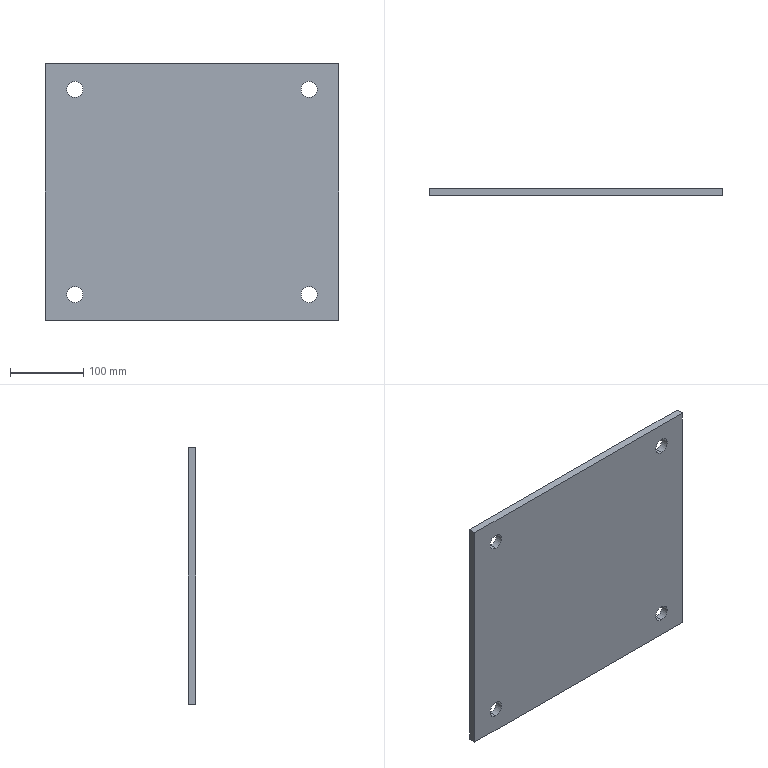Part | STEP file | 立柱Pad-400×350 | 1 solid | 14 faces | box 400 x 10 x 350 mm | volume 1384795 mm3 | cylinder 8 | plane 6 | commonest cylinder face diameters 22 x8
STEP:
#1=CARTESIAN_POINT('',(0.,0.,0.));
#2=DIRECTION('',(0.,0.,1.));
#3=DIRECTION('',(1.,0.,0.));
#4=AXIS2_PLACEMENT_3D('',#1,#2,#3);
#5=CARTESIAN_POINT('',(-160.,0.,-129.));
#6=VERTEX_POINT('',#5);
#7=CARTESIAN_POINT('',(-160.,10.,-129.));
#8=VERTEX_POINT('',#7);
#9=CARTESIAN_POINT('',(-160.,10.,-129.));
#10=DIRECTION('',(0.,1.,0.));
#11=VECTOR('',#10,1.);
#12=LINE('',#9,#11);
#13=CARTESIAN_POINT('',(-160.,10.,-140.));
#14=DIRECTION('',(0.,1.,0.));
#15=DIRECTION('',(0.,0.,1.));
#16=AXIS2_PLACEMENT_3D('',#13,#14,#15);
#17=CYLINDRICAL_SURFACE('',#16,11.);
#18=CARTESIAN_POINT('',(6.283,0.));
#19=DIRECTION('',(0.,1.));
#20=VECTOR('',#19,1.);
#21=LINE('',#18,#20);
#22=(GEOMETRIC_REPRESENTATION_CONTEXT(2)PARAMETRIC_REPRESENTATION_CONTEXT()REPRESENTATION_CONTEXT('',''));
#23=DEFINITIONAL_REPRESENTATION('',(#21),#22);
#24=PCURVE('',#17,#23);
#25=CARTESIAN_POINT('',(-160.,10.,-140.));
#26=DIRECTION('',(0.,1.,0.));
#27=DIRECTION('',(0.,0.,1.));
#28=AXIS2_PLACEMENT_3D('',#25,#26,#27);
#29=CYLINDRICAL_SURFACE('',#28,11.);
#30=CARTESIAN_POINT('',(0.,0.));
#31=DIRECTION('',(0.,1.));
#32=VECTOR('',#31,1.);
#33=LINE('',#30,#32);
#34=(GEOMETRIC_REPRESENTATION_CONTEXT(2)PARAMETRIC_REPRESENTATION_CONTEXT()REPRESENTATION_CONTEXT('',''));
#35=DEFINITIONAL_REPRESENTATION('',(#33),#34);
#36=PCURVE('',#29,#35);
#37=SURFACE_CURVE('',#12,(#24,#36),.PCURVE_S1.);
#38=EDGE_CURVE('',#6,#8,#37,.T.);
#39=ORIENTED_EDGE('',*,*,#38,.T.);
#40=CARTESIAN_POINT('',(-160.,10.,-151.));
#41=VERTEX_POINT('',#40);
#42=CARTESIAN_POINT('',(-160.,10.,-140.));
#43=DIRECTION('',(0.,1.,0.));
#44=DIRECTION('',(0.,0.,1.));
#45=AXIS2_PLACEMENT_3D('',#42,#43,#44);
#46=CIRCLE('',#45,11.);
#47=CARTESIAN_POINT('',(0.,0.));
#48=DIRECTION('',(1.,0.));
#49=VECTOR('',#48,1.);
#50=LINE('',#47,#49);
#51=(GEOMETRIC_REPRESENTATION_CONTEXT(2)PARAMETRIC_REPRESENTATION_CONTEXT()REPRESENTATION_CONTEXT('',''));
#52=DEFINITIONAL_REPRESENTATION('',(#50),#51);
#53=PCURVE('',#17,#52);
#54=CARTESIAN_POINT('',(0.,10.,0.));
#55=DIRECTION('',(0.,1.,0.));
#56=DIRECTION('',(0.,0.,1.));
#57=AXIS2_PLACEMENT_3D('',#54,#55,#56);
#58=PLANE('',#57);
#59=CARTESIAN_POINT('',(-140.,-160.));
#60=DIRECTION('',(1.,0.));
#61=AXIS2_PLACEMENT_2D('',#59,#60);
#62=CIRCLE('',#61,11.);
#63=(GEOMETRIC_REPRESENTATION_CONTEXT(2)PARAMETRIC_REPRESENTATION_CONTEXT()REPRESENTATION_CONTEXT('',''));
#64=DEFINITIONAL_REPRESENTATION('',(#62),#63);
#65=PCURVE('',#58,#64);
#66=SURFACE_CURVE('',#46,(#53,#65),.PCURVE_S1.);
#67=EDGE_CURVE('',#41,#8,#66,.T.);
#68=ORIENTED_EDGE('',*,*,#67,.F.);
#69=CARTESIAN_POINT('',(-160.,0.,-151.));
#70=VERTEX_POINT('',#69);
#71=CARTESIAN_POINT('',(-160.,10.,-151.));
#72=DIRECTION('',(0.,1.,0.));
#73=VECTOR('',#72,1.);
#74=LINE('',#71,#73);
#75=CARTESIAN_POINT('',(3.142,0.));
#76=DIRECTION('',(0.,1.));
#77=VECTOR('',#76,1.);
#78=LINE('',#75,#77);
#79=(GEOMETRIC_REPRESENTATION_CONTEXT(2)PARAMETRIC_REPRESENTATION_CONTEXT()REPRESENTATION_CONTEXT('',''));
#80=DEFINITIONAL_REPRESENTATION('',(#78),#79);
#81=PCURVE('',#17,#80);
#82=CARTESIAN_POINT('',(3.142,0.));
#83=DIRECTION('',(0.,1.));
#84=VECTOR('',#83,1.);
#85=LINE('',#82,#84);
#86=(GEOMETRIC_REPRESENTATION_CONTEXT(2)PARAMETRIC_REPRESENTATION_CONTEXT()REPRESENTATION_CONTEXT('',''));
#87=DEFINITIONAL_REPRESENTATION('',(#85),#86);
#88=PCURVE('',#29,#87);
#89=SURFACE_CURVE('',#74,(#81,#88),.PCURVE_S1.);
#90=EDGE_CURVE('',#70,#41,#89,.T.);
#91=ORIENTED_EDGE('',*,*,#90,.F.);
#92=CARTESIAN_POINT('',(-160.,0.,-140.));
#93=DIRECTION('',(0.,1.,0.));
#94=DIRECTION('',(0.,0.,1.));
#95=AXIS2_PLACEMENT_3D('',#92,#93,#94);
#96=CIRCLE('',#95,11.);
#97=CARTESIAN_POINT('',(0.,-10.));
#98=DIRECTION('',(1.,0.));
#99=VECTOR('',#98,1.);
#100=LINE('',#97,#99);
#101=(GEOMETRIC_REPRESENTATION_CONTEXT(2)PARAMETRIC_REPRESENTATION_CONTEXT()REPRESENTATION_CONTEXT('',''));
#102=DEFINITIONAL_REPRESENTATION('',(#100),#101);
#103=PCURVE('',#17,#102);
#104=CARTESIAN_POINT('',(0.,0.,0.));
#105=DIRECTION('',(0.,1.,0.));
#106=DIRECTION('',(0.,0.,1.));
#107=AXIS2_PLACEMENT_3D('',#104,#105,#106);
#108=PLANE('',#107);
#109=CARTESIAN_POINT('',(-140.,-160.));
#110=DIRECTION('',(1.,0.));
#111=AXIS2_PLACEMENT_2D('',#109,#110);
#112=CIRCLE('',#111,11.);
#113=(GEOMETRIC_REPRESENTATION_CONTEXT(2)PARAMETRIC_REPRESENTATION_CONTEXT()REPRESENTATION_CONTEXT('',''));
#114=DEFINITIONAL_REPRESENTATION('',(#112),#113);
#115=PCURVE('',#108,#114);
#116=SURFACE_CURVE('',#96,(#103,#115),.PCURVE_S1.);
#117=EDGE_CURVE('',#70,#6,#116,.T.);
#118=ORIENTED_EDGE('',*,*,#117,.T.);
#119=EDGE_LOOP('',(#39,#68,#91,#118));
#120=FACE_BOUND('',#119,.F.);
#121=ADVANCED_FACE('',(#120),#17,.F.);
#122=CARTESIAN_POINT('',(-160.,0.,151.));
#123=VERTEX_POINT('',#122);
#124=CARTESIAN_POINT('',(-160.,10.,151.));
#125=VERTEX_POINT('',#124);
#126=CARTESIAN_POINT('',(-160.,10.,151.));
#127=DIRECTION('',(0.,1.,0.));
#128=VECTOR('',#127,1.);
#129=LINE('',#126,#128);
#130=CARTESIAN_POINT('',(-160.,10.,140.));
#131=DIRECTION('',(0.,1.,0.));
#132=DIRECTION('',(0.,0.,1.));
#133=AXIS2_PLACEMENT_3D('',#130,#131,#132);
#134=CYLINDRICAL_SURFACE('',#133,11.);
#135=CARTESIAN_POINT('',(6.283,0.));
#136=DIRECTION('',(0.,1.));
#137=VECTOR('',#136,1.);
#138=LINE('',#135,#137);
#139=(GEOMETRIC_REPRESENTATION_CONTEXT(2)PARAMETRIC_REPRESENTATION_CONTEXT()REPRESENTATION_CONTEXT('',''));
#140=DEFINITIONAL_REPRESENTATION('',(#138),#139);
#141=PCURVE('',#134,#140);
#142=CARTESIAN_POINT('',(-160.,10.,140.));
#143=DIRECTION('',(0.,1.,0.));
#144=DIRECTION('',(0.,0.,1.));
#145=AXIS2_PLACEMENT_3D('',#142,#143,#144);
#146=CYLINDRICAL_SURFACE('',#145,11.);
#147=CARTESIAN_POINT('',(0.,0.));
#148=DIRECTION('',(0.,1.));
#149=VECTOR('',#148,1.);
#150=LINE('',#147,#149);
#151=(GEOMETRIC_REPRESENTATION_CONTEXT(2)PARAMETRIC_REPRESENTATION_CONTEXT()REPRESENTATION_CONTEXT('',''));
#152=DEFINITIONAL_REPRESENTATION('',(#150),#151);
#153=PCURVE('',#146,#152);
#154=SURFACE_CURVE('',#129,(#141,#153),.PCURVE_S1.);
#155=EDGE_CURVE('',#123,#125,#154,.T.);
#156=ORIENTED_EDGE('',*,*,#155,.T.);
#157=CARTESIAN_POINT('',(-160.,10.,129.));
#158=VERTEX_POINT('',#157);
#159=CARTESIAN_POINT('',(-160.,10.,140.));
#160=DIRECTION('',(0.,1.,0.));
#161=DIRECTION('',(0.,0.,1.));
#162=AXIS2_PLACEMENT_3D('',#159,#160,#161);
#163=CIRCLE('',#162,11.);
#164=CARTESIAN_POINT('',(0.,0.));
#165=DIRECTION('',(1.,0.));
#166=VECTOR('',#165,1.);
#167=LINE('',#164,#166);
#168=(GEOMETRIC_REPRESENTATION_CONTEXT(2)PARAMETRIC_REPRESENTATION_CONTEXT()REPRESENTATION_CONTEXT('',''));
#169=DEFINITIONAL_REPRESENTATION('',(#167),#168);
#170=PCURVE('',#134,#169);
#171=CARTESIAN_POINT('',(140.,-160.));
#172=DIRECTION('',(1.,0.));
#173=AXIS2_PLACEMENT_2D('',#171,#172);
#174=CIRCLE('',#173,11.);
#175=(GEOMETRIC_REPRESENTATION_CONTEXT(2)PARAMETRIC_REPRESENTATION_CONTEXT()REPRESENTATION_CONTEXT('',''));
#176=DEFINITIONAL_REPRESENTATION('',(#174),#175);
#177=PCURVE('',#58,#176);
#178=SURFACE_CURVE('',#163,(#170,#177),.PCURVE_S1.);
#179=EDGE_CURVE('',#158,#125,#178,.T.);
#180=ORIENTED_EDGE('',*,*,#179,.F.);
#181=CARTESIAN_POINT('',(-160.,0.,129.));
#182=VERTEX_POINT('',#181);
#183=CARTESIAN_POINT('',(-160.,10.,129.));
#184=DIRECTION('',(0.,1.,0.));
#185=VECTOR('',#184,1.);
#186=LINE('',#183,#185);
#187=CARTESIAN_POINT('',(3.142,0.));
#188=DIRECTION('',(0.,1.));
#189=VECTOR('',#188,1.);
#190=LINE('',#187,#189);
#191=(GEOMETRIC_REPRESENTATION_CONTEXT(2)PARAMETRIC_REPRESENTATION_CONTEXT()REPRESENTATION_CONTEXT('',''));
#192=DEFINITIONAL_REPRESENTATION('',(#190),#191);
#193=PCURVE('',#134,#192);
#194=CARTESIAN_POINT('',(3.142,0.));
#195=DIRECTION('',(0.,1.));
#196=VECTOR('',#195,1.);
#197=LINE('',#194,#196);
#198=(GEOMETRIC_REPRESENTATION_CONTEXT(2)PARAMETRIC_REPRESENTATION_CONTEXT()REPRESENTATION_CONTEXT('',''));
#199=DEFINITIONAL_REPRESENTATION('',(#197),#198);
#200=PCURVE('',#146,#199);
#201=SURFACE_CURVE('',#186,(#193,#200),.PCURVE_S1.);
#202=EDGE_CURVE('',#182,#158,#201,.T.);
#203=ORIENTED_EDGE('',*,*,#202,.F.);
#204=CARTESIAN_POINT('',(-160.,0.,140.));
#205=DIRECTION('',(0.,1.,0.));
#206=DIRECTION('',(0.,0.,1.));
#207=AXIS2_PLACEMENT_3D('',#204,#205,#206);
#208=CIRCLE('',#207,11.);
#209=CARTESIAN_POINT('',(0.,-10.));
#210=DIRECTION('',(1.,0.));
#211=VECTOR('',#210,1.);
#212=LINE('',#209,#211);
#213=(GEOMETRIC_REPRESENTATION_CONTEXT(2)PARAMETRIC_REPRESENTATION_CONTEXT()REPRESENTATION_CONTEXT('',''));
#214=DEFINITIONAL_REPRESENTATION('',(#212),#213);
#215=PCURVE('',#134,#214);
#216=CARTESIAN_POINT('',(140.,-160.));
#217=DIRECTION('',(1.,0.));
#218=AXIS2_PLACEMENT_2D('',#216,#217);
#219=CIRCLE('',#218,11.);
#220=(GEOMETRIC_REPRESENTATION_CONTEXT(2)PARAMETRIC_REPRESENTATION_CONTEXT()REPRESENTATION_CONTEXT('',''));
#221=DEFINITIONAL_REPRESENTATION('',(#219),#220);
#222=PCURVE('',#108,#221);
#223=SURFACE_CURVE('',#208,(#215,#222),.PCURVE_S1.);
#224=EDGE_CURVE('',#182,#123,#223,.T.);
#225=ORIENTED_EDGE('',*,*,#224,.T.);
#226=EDGE_LOOP('',(#156,#180,#203,#225));
#227=FACE_BOUND('',#226,.F.);
#228=ADVANCED_FACE('',(#227),#134,.F.);
#229=CARTESIAN_POINT('',(160.,0.,151.));
#230=VERTEX_POINT('',#229);
#231=CARTESIAN_POINT('',(160.,10.,151.));
#232=VERTEX_POINT('',#231);
#233=CARTESIAN_POINT('',(160.,10.,151.));
#234=DIRECTION('',(0.,1.,0.));
#235=VECTOR('',#234,1.);
#236=LINE('',#233,#235);
#237=CARTESIAN_POINT('',(160.,10.,140.));
#238=DIRECTION('',(0.,1.,0.));
#239=DIRECTION('',(0.,0.,1.));
#240=AXIS2_PLACEMENT_3D('',#237,#238,#239);
#241=CYLINDRICAL_SURFACE('',#240,11.);
#242=CARTESIAN_POINT('',(6.283,0.));
#243=DIRECTION('',(0.,1.));
#244=VECTOR('',#243,1.);
#245=LINE('',#242,#244);
#246=(GEOMETRIC_REPRESENTATION_CONTEXT(2)PARAMETRIC_REPRESENTATION_CONTEXT()REPRESENTATION_CONTEXT('',''));
#247=DEFINITIONAL_REPRESENTATION('',(#245),#246);
#248=PCURVE('',#241,#247);
#249=CARTESIAN_POINT('',(160.,10.,140.));
#250=DIRECTION('',(0.,1.,0.));
#251=DIRECTION('',(0.,0.,1.));
#252=AXIS2_PLACEMENT_3D('',#249,#250,#251);
#253=CYLINDRICAL_SURFACE('',#252,11.);
#254=CARTESIAN_POINT('',(0.,0.));
#255=DIRECTION('',(0.,1.));
#256=VECTOR('',#255,1.);
#257=LINE('',#254,#256);
#258=(GEOMETRIC_REPRESENTATION_CONTEXT(2)PARAMETRIC_REPRESENTATION_CONTEXT()REPRESENTATION_CONTEXT('',''));
#259=DEFINITIONAL_REPRESENTATION('',(#257),#258);
#260=PCURVE('',#253,#259);
#261=SURFACE_CURVE('',#236,(#248,#260),.PCURVE_S1.);
#262=EDGE_CURVE('',#230,#232,#261,.T.);
#263=ORIENTED_EDGE('',*,*,#262,.T.);
#264=CARTESIAN_POINT('',(160.,10.,129.));
#265=VERTEX_POINT('',#264);
#266=CARTESIAN_POINT('',(160.,10.,140.));
#267=DIRECTION('',(0.,1.,0.));
#268=DIRECTION('',(0.,0.,1.));
#269=AXIS2_PLACEMENT_3D('',#266,#267,#268);
#270=CIRCLE('',#269,11.);
#271=CARTESIAN_POINT('',(0.,0.));
#272=DIRECTION('',(1.,0.));
#273=VECTOR('',#272,1.);
#274=LINE('',#271,#273);
#275=(GEOMETRIC_REPRESENTATION_CONTEXT(2)PARAMETRIC_REPRESENTATION_CONTEXT()REPRESENTATION_CONTEXT('',''));
#276=DEFINITIONAL_REPRESENTATION('',(#274),#275);
#277=PCURVE('',#241,#276);
#278=CARTESIAN_POINT('',(140.,160.));
#279=DIRECTION('',(1.,0.));
#280=AXIS2_PLACEMENT_2D('',#278,#279);
#281=CIRCLE('',#280,11.);
#282=(GEOMETRIC_REPRESENTATION_CONTEXT(2)PARAMETRIC_REPRESENTATION_CONTEXT()REPRESENTATION_CONTEXT('',''));
#283=DEFINITIONAL_REPRESENTATION('',(#281),#282);
#284=PCURVE('',#58,#283);
#285=SURFACE_CURVE('',#270,(#277,#284),.PCURVE_S1.);
#286=EDGE_CURVE('',#265,#232,#285,.T.);
#287=ORIENTED_EDGE('',*,*,#286,.F.);
#288=CARTESIAN_POINT('',(160.,0.,129.));
#289=VERTEX_POINT('',#288);
#290=CARTESIAN_POINT('',(160.,10.,129.));
#291=DIRECTION('',(0.,1.,0.));
#292=VECTOR('',#291,1.);
#293=LINE('',#290,#292);
#294=CARTESIAN_POINT('',(3.142,0.));
#295=DIRECTION('',(0.,1.));
#296=VECTOR('',#295,1.);
#297=LINE('',#294,#296);
#298=(GEOMETRIC_REPRESENTATION_CONTEXT(2)PARAMETRIC_REPRESENTATION_CONTEXT()REPRESENTATION_CONTEXT('',''));
#299=DEFINITIONAL_REPRESENTATION('',(#297),#298);
#300=PCURVE('',#241,#299);
#301=CARTESIAN_POINT('',(3.142,0.));
#302=DIRECTION('',(0.,1.));
#303=VECTOR('',#302,1.);
#304=LINE('',#301,#303);
#305=(GEOMETRIC_REPRESENTATION_CONTEXT(2)PARAMETRIC_REPRESENTATION_CONTEXT()REPRESENTATION_CONTEXT('',''));
#306=DEFINITIONAL_REPRESENTATION('',(#304),#305);
#307=PCURVE('',#253,#306);
#308=SURFACE_CURVE('',#293,(#300,#307),.PCURVE_S1.);
#309=EDGE_CURVE('',#289,#265,#308,.T.);
#310=ORIENTED_EDGE('',*,*,#309,.F.);
#311=CARTESIAN_POINT('',(160.,0.,140.));
#312=DIRECTION('',(0.,1.,0.));
#313=DIRECTION('',(0.,0.,1.));
#314=AXIS2_PLACEMENT_3D('',#311,#312,#313);
#315=CIRCLE('',#314,11.);
#316=CARTESIAN_POINT('',(0.,-10.));
#317=DIRECTION('',(1.,0.));
#318=VECTOR('',#317,1.);
#319=LINE('',#316,#318);
#320=(GEOMETRIC_REPRESENTATION_CONTEXT(2)PARAMETRIC_REPRESENTATION_CONTEXT()REPRESENTATION_CONTEXT('',''));
#321=DEFINITIONAL_REPRESENTATION('',(#319),#320);
#322=PCURVE('',#241,#321);
#323=CARTESIAN_POINT('',(140.,160.));
#324=DIRECTION('',(1.,0.));
#325=AXIS2_PLACEMENT_2D('',#323,#324);
#326=CIRCLE('',#325,11.);
#327=(GEOMETRIC_REPRESENTATION_CONTEXT(2)PARAMETRIC_REPRESENTATION_CONTEXT()REPRESENTATION_CONTEXT('',''));
#328=DEFINITIONAL_REPRESENTATION('',(#326),#327);
#329=PCURVE('',#108,#328);
#330=SURFACE_CURVE('',#315,(#322,#329),.PCURVE_S1.);
#331=EDGE_CURVE('',#289,#230,#330,.T.);
#332=ORIENTED_EDGE('',*,*,#331,.T.);
#333=EDGE_LOOP('',(#263,#287,#310,#332));
#334=FACE_BOUND('',#333,.F.);
#335=ADVANCED_FACE('',(#334),#241,.F.);
#336=CARTESIAN_POINT('',(160.,0.,-129.));
#337=VERTEX_POINT('',#336);
#338=CARTESIAN_POINT('',(160.,10.,-129.));
#339=VERTEX_POINT('',#338);
#340=CARTESIAN_POINT('',(160.,10.,-129.));
#341=DIRECTION('',(0.,1.,0.));
#342=VECTOR('',#341,1.);
#343=LINE('',#340,#342);
#344=CARTESIAN_POINT('',(160.,10.,-140.));
#345=DIRECTION('',(0.,1.,0.));
#346=DIRECTION('',(0.,0.,1.));
#347=AXIS2_PLACEMENT_3D('',#344,#345,#346);
#348=CYLINDRICAL_SURFACE('',#347,11.);
#349=CARTESIAN_POINT('',(6.283,0.));
#350=DIRECTION('',(0.,1.));
#351=VECTOR('',#350,1.);
#352=LINE('',#349,#351);
#353=(GEOMETRIC_REPRESENTATION_CONTEXT(2)PARAMETRIC_REPRESENTATION_CONTEXT()REPRESENTATION_CONTEXT('',''));
#354=DEFINITIONAL_REPRESENTATION('',(#352),#353);
#355=PCURVE('',#348,#354);
#356=CARTESIAN_POINT('',(160.,10.,-140.));
#357=DIRECTION('',(0.,1.,0.));
#358=DIRECTION('',(0.,0.,1.));
#359=AXIS2_PLACEMENT_3D('',#356,#357,#358);
#360=CYLINDRICAL_SURFACE('',#359,11.);
#361=CARTESIAN_POINT('',(0.,0.));
#362=DIRECTION('',(0.,1.));
#363=VECTOR('',#362,1.);
#364=LINE('',#361,#363);
#365=(GEOMETRIC_REPRESENTATION_CONTEXT(2)PARAMETRIC_REPRESENTATION_CONTEXT()REPRESENTATION_CONTEXT('',''));
#366=DEFINITIONAL_REPRESENTATION('',(#364),#365);
#367=PCURVE('',#360,#366);
#368=SURFACE_CURVE('',#343,(#355,#367),.PCURVE_S1.);
#369=EDGE_CURVE('',#337,#339,#368,.T.);
#370=ORIENTED_EDGE('',*,*,#369,.T.);
#371=CARTESIAN_POINT('',(160.,10.,-151.));
#372=VERTEX_POINT('',#371);
#373=CARTESIAN_POINT('',(160.,10.,-140.));
#374=DIRECTION('',(0.,1.,0.));
#375=DIRECTION('',(0.,0.,1.));
#376=AXIS2_PLACEMENT_3D('',#373,#374,#375);
#377=CIRCLE('',#376,11.);
#378=CARTESIAN_POINT('',(0.,0.));
#379=DIRECTION('',(1.,0.));
#380=VECTOR('',#379,1.);
#381=LINE('',#378,#380);
#382=(GEOMETRIC_REPRESENTATION_CONTEXT(2)PARAMETRIC_REPRESENTATION_CONTEXT()REPRESENTATION_CONTEXT('',''));
#383=DEFINITIONAL_REPRESENTATION('',(#381),#382);
#384=PCURVE('',#348,#383);
#385=CARTESIAN_POINT('',(-140.,160.));
#386=DIRECTION('',(1.,0.));
#387=AXIS2_PLACEMENT_2D('',#385,#386);
#388=CIRCLE('',#387,11.);
#389=(GEOMETRIC_REPRESENTATION_CONTEXT(2)PARAMETRIC_REPRESENTATION_CONTEXT()REPRESENTATION_CONTEXT('',''));
#390=DEFINITIONAL_REPRESENTATION('',(#388),#389);
#391=PCURVE('',#58,#390);
#392=SURFACE_CURVE('',#377,(#384,#391),.PCURVE_S1.);
#393=EDGE_CURVE('',#372,#339,#392,.T.);
#394=ORIENTED_EDGE('',*,*,#393,.F.);
#395=CARTESIAN_POINT('',(160.,0.,-151.));
#396=VERTEX_POINT('',#395);
#397=CARTESIAN_POINT('',(160.,10.,-151.));
#398=DIRECTION('',(0.,1.,0.));
#399=VECTOR('',#398,1.);
#400=LINE('',#397,#399);
#401=CARTESIAN_POINT('',(3.142,0.));
#402=DIRECTION('',(0.,1.));
#403=VECTOR('',#402,1.);
#404=LINE('',#401,#403);
#405=(GEOMETRIC_REPRESENTATION_CONTEXT(2)PARAMETRIC_REPRESENTATION_CONTEXT()REPRESENTATION_CONTEXT('',''));
#406=DEFINITIONAL_REPRESENTATION('',(#404),#405);
#407=PCURVE('',#348,#406);
#408=CARTESIAN_POINT('',(3.142,0.));
#409=DIRECTION('',(0.,1.));
#410=VECTOR('',#409,1.);
#411=LINE('',#408,#410);
#412=(GEOMETRIC_REPRESENTATION_CONTEXT(2)PARAMETRIC_REPRESENTATION_CONTEXT()REPRESENTATION_CONTEXT('',''));
#413=DEFINITIONAL_REPRESENTATION('',(#411),#412);
#414=PCURVE('',#360,#413);
#415=SURFACE_CURVE('',#400,(#407,#414),.PCURVE_S1.);
#416=EDGE_CURVE('',#396,#372,#415,.T.);
#417=ORIENTED_EDGE('',*,*,#416,.F.);
#418=CARTESIAN_POINT('',(160.,0.,-140.));
#419=DIRECTION('',(0.,1.,0.));
#420=DIRECTION('',(0.,0.,1.));
#421=AXIS2_PLACEMENT_3D('',#418,#419,#420);
#422=CIRCLE('',#421,11.);
#423=CARTESIAN_POINT('',(0.,-10.));
#424=DIRECTION('',(1.,0.));
#425=VECTOR('',#424,1.);
#426=LINE('',#423,#425);
#427=(GEOMETRIC_REPRESENTATION_CONTEXT(2)PARAMETRIC_REPRESENTATION_CONTEXT()REPRESENTATION_CONTEXT('',''));
#428=DEFINITIONAL_REPRESENTATION('',(#426),#427);
#429=PCURVE('',#348,#428);
#430=CARTESIAN_POINT('',(-140.,160.));
#431=DIRECTION('',(1.,0.));
#432=AXIS2_PLACEMENT_2D('',#430,#431);
#433=CIRCLE('',#432,11.);
#434=(GEOMETRIC_REPRESENTATION_CONTEXT(2)PARAMETRIC_REPRESENTATION_CONTEXT()REPRESENTATION_CONTEXT('',''));
#435=DEFINITIONAL_REPRESENTATION('',(#433),#434);
#436=PCURVE('',#108,#435);
#437=SURFACE_CURVE('',#422,(#429,#436),.PCURVE_S1.);
#438=EDGE_CURVE('',#396,#337,#437,.T.);
#439=ORIENTED_EDGE('',*,*,#438,.T.);
#440=EDGE_LOOP('',(#370,#394,#417,#439));
#441=FACE_BOUND('',#440,.F.);
#442=ADVANCED_FACE('',(#441),#348,.F.);
#443=CARTESIAN_POINT('',(200.,0.,175.));
#444=VERTEX_POINT('',#443);
#445=CARTESIAN_POINT('',(200.,0.,-175.));
#446=VERTEX_POINT('',#445);
#447=CARTESIAN_POINT('',(200.,0.,-175.));
#448=DIRECTION('',(0.,0.,-1.));
#449=VECTOR('',#448,1.);
#450=LINE('',#447,#449);
#451=CARTESIAN_POINT('',(200.,10.,-175.));
#452=DIRECTION('',(-1.,0.,0.));
#453=DIRECTION('',(0.,0.,1.));
#454=AXIS2_PLACEMENT_3D('',#451,#452,#453);
#455=PLANE('',#454);
#456=CARTESIAN_POINT('',(0.,-10.));
#457=DIRECTION('',(-1.,0.));
#458=VECTOR('',#457,1.);
#459=LINE('',#456,#458);
#460=(GEOMETRIC_REPRESENTATION_CONTEXT(2)PARAMETRIC_REPRESENTATION_CONTEXT()REPRESENTATION_CONTEXT('',''));
#461=DEFINITIONAL_REPRESENTATION('',(#459),#460);
#462=PCURVE('',#455,#461);
#463=CARTESIAN_POINT('',(-175.,200.));
#464=DIRECTION('',(-1.,0.));
#465=VECTOR('',#464,1.);
#466=LINE('',#463,#465);
#467=(GEOMETRIC_REPRESENTATION_CONTEXT(2)PARAMETRIC_REPRESENTATION_CONTEXT()REPRESENTATION_CONTEXT('',''));
#468=DEFINITIONAL_REPRESENTATION('',(#466),#467);
#469=PCURVE('',#108,#468);
#470=SURFACE_CURVE('',#450,(#462,#469),.PCURVE_S1.);
#471=EDGE_CURVE('',#444,#446,#470,.T.);
#472=ORIENTED_EDGE('',*,*,#471,.T.);
#473=CARTESIAN_POINT('',(200.,10.,-175.));
#474=VERTEX_POINT('',#473);
#475=CARTESIAN_POINT('',(200.,10.,-175.));
#476=DIRECTION('',(0.,-1.,0.));
#477=VECTOR('',#476,1.);
#478=LINE('',#475,#477);
#479=CARTESIAN_POINT('',(0.,0.));
#480=DIRECTION('',(0.,-1.));
#481=VECTOR('',#480,1.);
#482=LINE('',#479,#481);
#483=(GEOMETRIC_REPRESENTATION_CONTEXT(2)PARAMETRIC_REPRESENTATION_CONTEXT()REPRESENTATION_CONTEXT('',''));
#484=DEFINITIONAL_REPRESENTATION('',(#482),#483);
#485=PCURVE('',#455,#484);
#486=CARTESIAN_POINT('',(-200.,10.,-175.));
#487=DIRECTION('',(0.,0.,1.));
#488=DIRECTION('',(1.,0.,0.));
#489=AXIS2_PLACEMENT_3D('',#486,#487,#488);
#490=PLANE('',#489);
#491=CARTESIAN_POINT('',(400.,0.));
#492=DIRECTION('',(0.,-1.));
#493=VECTOR('',#492,1.);
#494=LINE('',#491,#493);
#495=(GEOMETRIC_REPRESENTATION_CONTEXT(2)PARAMETRIC_REPRESENTATION_CONTEXT()REPRESENTATION_CONTEXT('',''));
#496=DEFINITIONAL_REPRESENTATION('',(#494),#495);
#497=PCURVE('',#490,#496);
#498=SURFACE_CURVE('',#478,(#485,#497),.PCURVE_S1.);
#499=EDGE_CURVE('',#474,#446,#498,.T.);
#500=ORIENTED_EDGE('',*,*,#499,.F.);
#501=CARTESIAN_POINT('',(200.,10.,175.));
#502=VERTEX_POINT('',#501);
#503=CARTESIAN_POINT('',(200.,10.,-175.));
#504=DIRECTION('',(0.,0.,-1.));
#505=VECTOR('',#504,1.);
#506=LINE('',#503,#505);
#507=CARTESIAN_POINT('',(0.,0.));
#508=DIRECTION('',(-1.,0.));
#509=VECTOR('',#508,1.);
#510=LINE('',#507,#509);
#511=(GEOMETRIC_REPRESENTATION_CONTEXT(2)PARAMETRIC_REPRESENTATION_CONTEXT()REPRESENTATION_CONTEXT('',''));
#512=DEFINITIONAL_REPRESENTATION('',(#510),#511);
#513=PCURVE('',#455,#512);
#514=CARTESIAN_POINT('',(-175.,200.));
#515=DIRECTION('',(-1.,0.));
#516=VECTOR('',#515,1.);
#517=LINE('',#514,#516);
#518=(GEOMETRIC_REPRESENTATION_CONTEXT(2)PARAMETRIC_REPRESENTATION_CONTEXT()REPRESENTATION_CONTEXT('',''));
#519=DEFINITIONAL_REPRESENTATION('',(#517),#518);
#520=PCURVE('',#58,#519);
#521=SURFACE_CURVE('',#506,(#513,#520),.PCURVE_S1.);
#522=EDGE_CURVE('',#502,#474,#521,.T.);
#523=ORIENTED_EDGE('',*,*,#522,.F.);
#524=CARTESIAN_POINT('',(200.,10.,175.));
#525=DIRECTION('',(0.,-1.,0.));
#526=VECTOR('',#525,1.);
#527=LINE('',#524,#526);
#528=CARTESIAN_POINT('',(350.,0.));
#529=DIRECTION('',(0.,-1.));
#530=VECTOR('',#529,1.);
#531=LINE('',#528,#530);
#532=(GEOMETRIC_REPRESENTATION_CONTEXT(2)PARAMETRIC_REPRESENTATION_CONTEXT()REPRESENTATION_CONTEXT('',''));
#533=DEFINITIONAL_REPRESENTATION('',(#531),#532);
#534=PCURVE('',#455,#533);
#535=CARTESIAN_POINT('',(-200.,10.,175.));
#536=DIRECTION('',(0.,0.,-1.));
#537=DIRECTION('',(-1.,0.,0.));
#538=AXIS2_PLACEMENT_3D('',#535,#536,#537);
#539=PLANE('',#538);
#540=CARTESIAN_POINT('',(-400.,0.));
#541=DIRECTION('',(0.,-1.));
#542=VECTOR('',#541,1.);
#543=LINE('',#540,#542);
#544=(GEOMETRIC_REPRESENTATION_CONTEXT(2)PARAMETRIC_REPRESENTATION_CONTEXT()REPRESENTATION_CONTEXT('',''));
#545=DEFINITIONAL_REPRESENTATION('',(#543),#544);
#546=PCURVE('',#539,#545);
#547=SURFACE_CURVE('',#527,(#534,#546),.PCURVE_S1.);
#548=EDGE_CURVE('',#502,#444,#547,.T.);
#549=ORIENTED_EDGE('',*,*,#548,.T.);
#550=EDGE_LOOP('',(#472,#500,#523,#549));
#551=FACE_BOUND('',#550,.T.);
#552=ADVANCED_FACE('',(#551),#455,.F.);
#553=CARTESIAN_POINT('',(-200.,0.,-175.));
#554=VERTEX_POINT('',#553);
#555=CARTESIAN_POINT('',(-200.,0.,-175.));
#556=DIRECTION('',(-1.,0.,0.));
#557=VECTOR('',#556,1.);
#558=LINE('',#555,#557);
#559=CARTESIAN_POINT('',(0.,-10.));
#560=DIRECTION('',(-1.,0.));
#561=VECTOR('',#560,1.);
#562=LINE('',#559,#561);
#563=(GEOMETRIC_REPRESENTATION_CONTEXT(2)PARAMETRIC_REPRESENTATION_CONTEXT()REPRESENTATION_CONTEXT('',''));
#564=DEFINITIONAL_REPRESENTATION('',(#562),#563);
#565=PCURVE('',#490,#564);
#566=CARTESIAN_POINT('',(-175.,-200.));
#567=DIRECTION('',(0.,-1.));
#568=VECTOR('',#567,1.);
#569=LINE('',#566,#568);
#570=(GEOMETRIC_REPRESENTATION_CONTEXT(2)PARAMETRIC_REPRESENTATION_CONTEXT()REPRESENTATION_CONTEXT('',''));
#571=DEFINITIONAL_REPRESENTATION('',(#569),#570);
#572=PCURVE('',#108,#571);
#573=SURFACE_CURVE('',#558,(#565,#572),.PCURVE_S1.);
#574=EDGE_CURVE('',#446,#554,#573,.T.);
#575=ORIENTED_EDGE('',*,*,#574,.T.);
#576=CARTESIAN_POINT('',(-200.,10.,-175.));
#577=VERTEX_POINT('',#576);
#578=CARTESIAN_POINT('',(-200.,10.,-175.));
#579=DIRECTION('',(0.,-1.,0.));
#580=VECTOR('',#579,1.);
#581=LINE('',#578,#580);
#582=CARTESIAN_POINT('',(0.,0.));
#583=DIRECTION('',(0.,-1.));
#584=VECTOR('',#583,1.);
#585=LINE('',#582,#584);
#586=(GEOMETRIC_REPRESENTATION_CONTEXT(2)PARAMETRIC_REPRESENTATION_CONTEXT()REPRESENTATION_CONTEXT('',''));
#587=DEFINITIONAL_REPRESENTATION('',(#585),#586);
#588=PCURVE('',#490,#587);
#589=CARTESIAN_POINT('',(-200.,10.,-175.));
#590=DIRECTION('',(1.,0.,0.));
#591=DIRECTION('',(0.,0.,-1.));
#592=AXIS2_PLACEMENT_3D('',#589,#590,#591);
#593=PLANE('',#592);
#594=CARTESIAN_POINT('',(0.,0.));
#595=DIRECTION('',(0.,-1.));
#596=VECTOR('',#595,1.);
#597=LINE('',#594,#596);
#598=(GEOMETRIC_REPRESENTATION_CONTEXT(2)PARAMETRIC_REPRESENTATION_CONTEXT()REPRESENTATION_CONTEXT('',''));
#599=DEFINITIONAL_REPRESENTATION('',(#597),#598);
#600=PCURVE('',#593,#599);
#601=SURFACE_CURVE('',#581,(#588,#600),.PCURVE_S1.);
#602=EDGE_CURVE('',#577,#554,#601,.T.);
#603=ORIENTED_EDGE('',*,*,#602,.F.);
#604=CARTESIAN_POINT('',(-200.,10.,-175.));
#605=DIRECTION('',(-1.,0.,0.));
#606=VECTOR('',#605,1.);
#607=LINE('',#604,#606);
#608=CARTESIAN_POINT('',(0.,0.));
#609=DIRECTION('',(-1.,0.));
#610=VECTOR('',#609,1.);
#611=LINE('',#608,#610);
#612=(GEOMETRIC_REPRESENTATION_CONTEXT(2)PARAMETRIC_REPRESENTATION_CONTEXT()REPRESENTATION_CONTEXT('',''));
#613=DEFINITIONAL_REPRESENTATION('',(#611),#612);
#614=PCURVE('',#490,#613);
#615=CARTESIAN_POINT('',(-175.,-200.));
#616=DIRECTION('',(0.,-1.));
#617=VECTOR('',#616,1.);
#618=LINE('',#615,#617);
#619=(GEOMETRIC_REPRESENTATION_CONTEXT(2)PARAMETRIC_REPRESENTATION_CONTEXT()REPRESENTATION_CONTEXT('',''));
#620=DEFINITIONAL_REPRESENTATION('',(#618),#619);
#621=PCURVE('',#58,#620);
#622=SURFACE_CURVE('',#607,(#614,#621),.PCURVE_S1.);
#623=EDGE_CURVE('',#474,#577,#622,.T.);
#624=ORIENTED_EDGE('',*,*,#623,.F.);
#625=ORIENTED_EDGE('',*,*,#499,.T.);
#626=EDGE_LOOP('',(#575,#603,#624,#625));
#627=FACE_BOUND('',#626,.T.);
#628=ADVANCED_FACE('',(#627),#490,.F.);
#629=CARTESIAN_POINT('',(-200.,0.,175.));
#630=VERTEX_POINT('',#629);
#631=CARTESIAN_POINT('',(-200.,0.,-175.));
#632=DIRECTION('',(0.,0.,1.));
#633=VECTOR('',#632,1.);
#634=LINE('',#631,#633);
#635=CARTESIAN_POINT('',(0.,-10.));
#636=DIRECTION('',(-1.,0.));
#637=VECTOR('',#636,1.);
#638=LINE('',#635,#637);
#639=(GEOMETRIC_REPRESENTATION_CONTEXT(2)PARAMETRIC_REPRESENTATION_CONTEXT()REPRESENTATION_CONTEXT('',''));
#640=DEFINITIONAL_REPRESENTATION('',(#638),#639);
#641=PCURVE('',#593,#640);
#642=CARTESIAN_POINT('',(-175.,-200.));
#643=DIRECTION('',(1.,0.));
#644=VECTOR('',#643,1.);
#645=LINE('',#642,#644);
#646=(GEOMETRIC_REPRESENTATION_CONTEXT(2)PARAMETRIC_REPRESENTATION_CONTEXT()REPRESENTATION_CONTEXT('',''));
#647=DEFINITIONAL_REPRESENTATION('',(#645),#646);
#648=PCURVE('',#108,#647);
#649=SURFACE_CURVE('',#634,(#641,#648),.PCURVE_S1.);
#650=EDGE_CURVE('',#554,#630,#649,.T.);
#651=ORIENTED_EDGE('',*,*,#650,.T.);
#652=CARTESIAN_POINT('',(-200.,10.,175.));
#653=VERTEX_POINT('',#652);
#654=CARTESIAN_POINT('',(-200.,10.,175.));
#655=DIRECTION('',(0.,-1.,0.));
#656=VECTOR('',#655,1.);
#657=LINE('',#654,#656);
#658=CARTESIAN_POINT('',(-350.,0.));
#659=DIRECTION('',(0.,-1.));
#660=VECTOR('',#659,1.);
#661=LINE('',#658,#660);
#662=(GEOMETRIC_REPRESENTATION_CONTEXT(2)PARAMETRIC_REPRESENTATION_CONTEXT()REPRESENTATION_CONTEXT('',''));
#663=DEFINITIONAL_REPRESENTATION('',(#661),#662);
#664=PCURVE('',#593,#663);
#665=CARTESIAN_POINT('',(0.,0.));
#666=DIRECTION('',(0.,-1.));
#667=VECTOR('',#666,1.);
#668=LINE('',#665,#667);
#669=(GEOMETRIC_REPRESENTATION_CONTEXT(2)PARAMETRIC_REPRESENTATION_CONTEXT()REPRESENTATION_CONTEXT('',''));
#670=DEFINITIONAL_REPRESENTATION('',(#668),#669);
#671=PCURVE('',#539,#670);
#672=SURFACE_CURVE('',#657,(#664,#671),.PCURVE_S1.);
#673=EDGE_CURVE('',#653,#630,#672,.T.);
#674=ORIENTED_EDGE('',*,*,#673,.F.);
#675=CARTESIAN_POINT('',(-200.,10.,-175.));
#676=DIRECTION('',(0.,0.,1.));
#677=VECTOR('',#676,1.);
#678=LINE('',#675,#677);
#679=CARTESIAN_POINT('',(0.,0.));
#680=DIRECTION('',(-1.,0.));
#681=VECTOR('',#680,1.);
#682=LINE('',#679,#681);
#683=(GEOMETRIC_REPRESENTATION_CONTEXT(2)PARAMETRIC_REPRESENTATION_CONTEXT()REPRESENTATION_CONTEXT('',''));
#684=DEFINITIONAL_REPRESENTATION('',(#682),#683);
#685=PCURVE('',#593,#684);
#686=CARTESIAN_POINT('',(-175.,-200.));
#687=DIRECTION('',(1.,0.));
#688=VECTOR('',#687,1.);
#689=LINE('',#686,#688);
#690=(GEOMETRIC_REPRESENTATION_CONTEXT(2)PARAMETRIC_REPRESENTATION_CONTEXT()REPRESENTATION_CONTEXT('',''));
#691=DEFINITIONAL_REPRESENTATION('',(#689),#690);
#692=PCURVE('',#58,#691);
#693=SURFACE_CURVE('',#678,(#685,#692),.PCURVE_S1.);
#694=EDGE_CURVE('',#577,#653,#693,.T.);
#695=ORIENTED_EDGE('',*,*,#694,.F.);
#696=ORIENTED_EDGE('',*,*,#602,.T.);
#697=EDGE_LOOP('',(#651,#674,#695,#696));
#698=FACE_BOUND('',#697,.T.);
#699=ADVANCED_FACE('',(#698),#593,.F.);
#700=CARTESIAN_POINT('',(-200.,0.,175.));
#701=DIRECTION('',(1.,0.,0.));
#702=VECTOR('',#701,1.);
#703=LINE('',#700,#702);
#704=CARTESIAN_POINT('',(0.,-10.));
#705=DIRECTION('',(-1.,0.));
#706=VECTOR('',#705,1.);
#707=LINE('',#704,#706);
#708=(GEOMETRIC_REPRESENTATION_CONTEXT(2)PARAMETRIC_REPRESENTATION_CONTEXT()REPRESENTATION_CONTEXT('',''));
#709=DEFINITIONAL_REPRESENTATION('',(#707),#708);
#710=PCURVE('',#539,#709);
#711=CARTESIAN_POINT('',(175.,-200.));
#712=DIRECTION('',(0.,1.));
#713=VECTOR('',#712,1.);
#714=LINE('',#711,#713);
#715=(GEOMETRIC_REPRESENTATION_CONTEXT(2)PARAMETRIC_REPRESENTATION_CONTEXT()REPRESENTATION_CONTEXT('',''));
#716=DEFINITIONAL_REPRESENTATION('',(#714),#715);
#717=PCURVE('',#108,#716);
#718=SURFACE_CURVE('',#703,(#710,#717),.PCURVE_S1.);
#719=EDGE_CURVE('',#630,#444,#718,.T.);
#720=ORIENTED_EDGE('',*,*,#719,.T.);
#721=ORIENTED_EDGE('',*,*,#548,.F.);
#722=CARTESIAN_POINT('',(-200.,10.,175.));
#723=DIRECTION('',(1.,0.,0.));
#724=VECTOR('',#723,1.);
#725=LINE('',#722,#724);
#726=CARTESIAN_POINT('',(0.,0.));
#727=DIRECTION('',(-1.,0.));
#728=VECTOR('',#727,1.);
#729=LINE('',#726,#728);
#730=(GEOMETRIC_REPRESENTATION_CONTEXT(2)PARAMETRIC_REPRESENTATION_CONTEXT()REPRESENTATION_CONTEXT('',''));
#731=DEFINITIONAL_REPRESENTATION('',(#729),#730);
#732=PCURVE('',#539,#731);
#733=CARTESIAN_POINT('',(175.,-200.));
#734=DIRECTION('',(0.,1.));
#735=VECTOR('',#734,1.);
#736=LINE('',#733,#735);
#737=(GEOMETRIC_REPRESENTATION_CONTEXT(2)PARAMETRIC_REPRESENTATION_CONTEXT()REPRESENTATION_CONTEXT('',''));
#738=DEFINITIONAL_REPRESENTATION('',(#736),#737);
#739=PCURVE('',#58,#738);
#740=SURFACE_CURVE('',#725,(#732,#739),.PCURVE_S1.);
#741=EDGE_CURVE('',#653,#502,#740,.T.);
#742=ORIENTED_EDGE('',*,*,#741,.F.);
#743=ORIENTED_EDGE('',*,*,#673,.T.);
#744=EDGE_LOOP('',(#720,#721,#742,#743));
#745=FACE_BOUND('',#744,.T.);
#746=ADVANCED_FACE('',(#745),#539,.F.);
#747=CARTESIAN_POINT('',(-160.,10.,-140.));
#748=DIRECTION('',(0.,1.,0.));
#749=DIRECTION('',(0.,0.,1.));
#750=AXIS2_PLACEMENT_3D('',#747,#748,#749);
#751=CIRCLE('',#750,11.);
#752=CARTESIAN_POINT('',(-140.,-160.));
#753=DIRECTION('',(1.,0.));
#754=AXIS2_PLACEMENT_2D('',#752,#753);
#755=CIRCLE('',#754,11.);
#756=(GEOMETRIC_REPRESENTATION_CONTEXT(2)PARAMETRIC_REPRESENTATION_CONTEXT()REPRESENTATION_CONTEXT('',''));
#757=DEFINITIONAL_REPRESENTATION('',(#755),#756);
#758=PCURVE('',#58,#757);
#759=CARTESIAN_POINT('',(0.,0.));
#760=DIRECTION('',(1.,0.));
#761=VECTOR('',#760,1.);
#762=LINE('',#759,#761);
#763=(GEOMETRIC_REPRESENTATION_CONTEXT(2)PARAMETRIC_REPRESENTATION_CONTEXT()REPRESENTATION_CONTEXT('',''));
#764=DEFINITIONAL_REPRESENTATION('',(#762),#763);
#765=PCURVE('',#29,#764);
#766=SURFACE_CURVE('',#751,(#758,#765),.PCURVE_S1.);
#767=EDGE_CURVE('',#8,#41,#766,.T.);
#768=ORIENTED_EDGE('',*,*,#767,.F.);
#769=ORIENTED_EDGE('',*,*,#67,.F.);
#770=EDGE_LOOP('',(#768,#769));
#771=FACE_BOUND('',#770,.T.);
#772=CARTESIAN_POINT('',(-160.,10.,140.));
#773=DIRECTION('',(0.,1.,0.));
#774=DIRECTION('',(0.,0.,1.));
#775=AXIS2_PLACEMENT_3D('',#772,#773,#774);
#776=CIRCLE('',#775,11.);
#777=CARTESIAN_POINT('',(140.,-160.));
#778=DIRECTION('',(1.,0.));
#779=AXIS2_PLACEMENT_2D('',#777,#778);
#780=CIRCLE('',#779,11.);
#781=(GEOMETRIC_REPRESENTATION_CONTEXT(2)PARAMETRIC_REPRESENTATION_CONTEXT()REPRESENTATION_CONTEXT('',''));
#782=DEFINITIONAL_REPRESENTATION('',(#780),#781);
#783=PCURVE('',#58,#782);
#784=CARTESIAN_POINT('',(0.,0.));
#785=DIRECTION('',(1.,0.));
#786=VECTOR('',#785,1.);
#787=LINE('',#784,#786);
#788=(GEOMETRIC_REPRESENTATION_CONTEXT(2)PARAMETRIC_REPRESENTATION_CONTEXT()REPRESENTATION_CONTEXT('',''));
#789=DEFINITIONAL_REPRESENTATION('',(#787),#788);
#790=PCURVE('',#146,#789);
#791=SURFACE_CURVE('',#776,(#783,#790),.PCURVE_S1.);
#792=EDGE_CURVE('',#125,#158,#791,.T.);
#793=ORIENTED_EDGE('',*,*,#792,.F.);
#794=ORIENTED_EDGE('',*,*,#179,.F.);
#795=EDGE_LOOP('',(#793,#794));
#796=FACE_BOUND('',#795,.T.);
#797=CARTESIAN_POINT('',(160.,10.,140.));
#798=DIRECTION('',(0.,1.,0.));
#799=DIRECTION('',(0.,0.,1.));
#800=AXIS2_PLACEMENT_3D('',#797,#798,#799);
#801=CIRCLE('',#800,11.);
#802=CARTESIAN_POINT('',(140.,160.));
#803=DIRECTION('',(1.,0.));
#804=AXIS2_PLACEMENT_2D('',#802,#803);
#805=CIRCLE('',#804,11.);
#806=(GEOMETRIC_REPRESENTATION_CONTEXT(2)PARAMETRIC_REPRESENTATION_CONTEXT()REPRESENTATION_CONTEXT('',''));
#807=DEFINITIONAL_REPRESENTATION('',(#805),#806);
#808=PCURVE('',#58,#807);
#809=CARTESIAN_POINT('',(0.,0.));
#810=DIRECTION('',(1.,0.));
#811=VECTOR('',#810,1.);
#812=LINE('',#809,#811);
#813=(GEOMETRIC_REPRESENTATION_CONTEXT(2)PARAMETRIC_REPRESENTATION_CONTEXT()REPRESENTATION_CONTEXT('',''));
#814=DEFINITIONAL_REPRESENTATION('',(#812),#813);
#815=PCURVE('',#253,#814);
#816=SURFACE_CURVE('',#801,(#808,#815),.PCURVE_S1.);
#817=EDGE_CURVE('',#232,#265,#816,.T.);
#818=ORIENTED_EDGE('',*,*,#817,.F.);
#819=ORIENTED_EDGE('',*,*,#286,.F.);
#820=EDGE_LOOP('',(#818,#819));
#821=FACE_BOUND('',#820,.T.);
#822=CARTESIAN_POINT('',(160.,10.,-140.));
#823=DIRECTION('',(0.,1.,0.));
#824=DIRECTION('',(0.,0.,1.));
#825=AXIS2_PLACEMENT_3D('',#822,#823,#824);
#826=CIRCLE('',#825,11.);
#827=CARTESIAN_POINT('',(-140.,160.));
#828=DIRECTION('',(1.,0.));
#829=AXIS2_PLACEMENT_2D('',#827,#828);
#830=CIRCLE('',#829,11.);
#831=(GEOMETRIC_REPRESENTATION_CONTEXT(2)PARAMETRIC_REPRESENTATION_CONTEXT()REPRESENTATION_CONTEXT('',''));
#832=DEFINITIONAL_REPRESENTATION('',(#830),#831);
#833=PCURVE('',#58,#832);
#834=CARTESIAN_POINT('',(0.,0.));
#835=DIRECTION('',(1.,0.));
#836=VECTOR('',#835,1.);
#837=LINE('',#834,#836);
#838=(GEOMETRIC_REPRESENTATION_CONTEXT(2)PARAMETRIC_REPRESENTATION_CONTEXT()REPRESENTATION_CONTEXT('',''));
#839=DEFINITIONAL_REPRESENTATION('',(#837),#838);
#840=PCURVE('',#360,#839);
#841=SURFACE_CURVE('',#826,(#833,#840),.PCURVE_S1.);
#842=EDGE_CURVE('',#339,#372,#841,.T.);
#843=ORIENTED_EDGE('',*,*,#842,.F.);
#844=ORIENTED_EDGE('',*,*,#393,.F.);
#845=EDGE_LOOP('',(#843,#844));
#846=FACE_BOUND('',#845,.T.);
#847=ORIENTED_EDGE('',*,*,#522,.T.);
#848=ORIENTED_EDGE('',*,*,#623,.T.);
#849=ORIENTED_EDGE('',*,*,#694,.T.);
#850=ORIENTED_EDGE('',*,*,#741,.T.);
#851=EDGE_LOOP('',(#847,#848,#849,#850));
#852=FACE_BOUND('',#851,.T.);
#853=ADVANCED_FACE('',(#771,#796,#821,#846,#852),#58,.T.);
#854=CARTESIAN_POINT('',(-160.,0.,-140.));
#855=DIRECTION('',(0.,1.,0.));
#856=DIRECTION('',(0.,0.,1.));
#857=AXIS2_PLACEMENT_3D('',#854,#855,#856);
#858=CIRCLE('',#857,11.);
#859=CARTESIAN_POINT('',(-140.,-160.));
#860=DIRECTION('',(1.,0.));
#861=AXIS2_PLACEMENT_2D('',#859,#860);
#862=CIRCLE('',#861,11.);
#863=(GEOMETRIC_REPRESENTATION_CONTEXT(2)PARAMETRIC_REPRESENTATION_CONTEXT()REPRESENTATION_CONTEXT('',''));
#864=DEFINITIONAL_REPRESENTATION('',(#862),#863);
#865=PCURVE('',#108,#864);
#866=CARTESIAN_POINT('',(0.,-10.));
#867=DIRECTION('',(1.,0.));
#868=VECTOR('',#867,1.);
#869=LINE('',#866,#868);
#870=(GEOMETRIC_REPRESENTATION_CONTEXT(2)PARAMETRIC_REPRESENTATION_CONTEXT()REPRESENTATION_CONTEXT('',''));
#871=DEFINITIONAL_REPRESENTATION('',(#869),#870);
#872=PCURVE('',#29,#871);
#873=SURFACE_CURVE('',#858,(#865,#872),.PCURVE_S1.);
#874=EDGE_CURVE('',#6,#70,#873,.T.);
#875=ORIENTED_EDGE('',*,*,#874,.T.);
#876=ORIENTED_EDGE('',*,*,#117,.T.);
#877=EDGE_LOOP('',(#875,#876));
#878=FACE_BOUND('',#877,.T.);
#879=CARTESIAN_POINT('',(-160.,0.,140.));
#880=DIRECTION('',(0.,1.,0.));
#881=DIRECTION('',(0.,0.,1.));
#882=AXIS2_PLACEMENT_3D('',#879,#880,#881);
#883=CIRCLE('',#882,11.);
#884=CARTESIAN_POINT('',(140.,-160.));
#885=DIRECTION('',(1.,0.));
#886=AXIS2_PLACEMENT_2D('',#884,#885);
#887=CIRCLE('',#886,11.);
#888=(GEOMETRIC_REPRESENTATION_CONTEXT(2)PARAMETRIC_REPRESENTATION_CONTEXT()REPRESENTATION_CONTEXT('',''));
#889=DEFINITIONAL_REPRESENTATION('',(#887),#888);
#890=PCURVE('',#108,#889);
#891=CARTESIAN_POINT('',(0.,-10.));
#892=DIRECTION('',(1.,0.));
#893=VECTOR('',#892,1.);
#894=LINE('',#891,#893);
#895=(GEOMETRIC_REPRESENTATION_CONTEXT(2)PARAMETRIC_REPRESENTATION_CONTEXT()REPRESENTATION_CONTEXT('',''));
#896=DEFINITIONAL_REPRESENTATION('',(#894),#895);
#897=PCURVE('',#146,#896);
#898=SURFACE_CURVE('',#883,(#890,#897),.PCURVE_S1.);
#899=EDGE_CURVE('',#123,#182,#898,.T.);
#900=ORIENTED_EDGE('',*,*,#899,.T.);
#901=ORIENTED_EDGE('',*,*,#224,.T.);
#902=EDGE_LOOP('',(#900,#901));
#903=FACE_BOUND('',#902,.T.);
#904=CARTESIAN_POINT('',(160.,0.,140.));
#905=DIRECTION('',(0.,1.,0.));
#906=DIRECTION('',(0.,0.,1.));
#907=AXIS2_PLACEMENT_3D('',#904,#905,#906);
#908=CIRCLE('',#907,11.);
#909=CARTESIAN_POINT('',(140.,160.));
#910=DIRECTION('',(1.,0.));
#911=AXIS2_PLACEMENT_2D('',#909,#910);
#912=CIRCLE('',#911,11.);
#913=(GEOMETRIC_REPRESENTATION_CONTEXT(2)PARAMETRIC_REPRESENTATION_CONTEXT()REPRESENTATION_CONTEXT('',''));
#914=DEFINITIONAL_REPRESENTATION('',(#912),#913);
#915=PCURVE('',#108,#914);
#916=CARTESIAN_POINT('',(0.,-10.));
#917=DIRECTION('',(1.,0.));
#918=VECTOR('',#917,1.);
#919=LINE('',#916,#918);
#920=(GEOMETRIC_REPRESENTATION_CONTEXT(2)PARAMETRIC_REPRESENTATION_CONTEXT()REPRESENTATION_CONTEXT('',''));
#921=DEFINITIONAL_REPRESENTATION('',(#919),#920);
#922=PCURVE('',#253,#921);
#923=SURFACE_CURVE('',#908,(#915,#922),.PCURVE_S1.);
#924=EDGE_CURVE('',#230,#289,#923,.T.);
#925=ORIENTED_EDGE('',*,*,#924,.T.);
#926=ORIENTED_EDGE('',*,*,#331,.T.);
#927=EDGE_LOOP('',(#925,#926));
#928=FACE_BOUND('',#927,.T.);
#929=CARTESIAN_POINT('',(160.,0.,-140.));
#930=DIRECTION('',(0.,1.,0.));
#931=DIRECTION('',(0.,0.,1.));
#932=AXIS2_PLACEMENT_3D('',#929,#930,#931);
#933=CIRCLE('',#932,11.);
#934=CARTESIAN_POINT('',(-140.,160.));
#935=DIRECTION('',(1.,0.));
#936=AXIS2_PLACEMENT_2D('',#934,#935);
#937=CIRCLE('',#936,11.);
#938=(GEOMETRIC_REPRESENTATION_CONTEXT(2)PARAMETRIC_REPRESENTATION_CONTEXT()REPRESENTATION_CONTEXT('',''));
#939=DEFINITIONAL_REPRESENTATION('',(#937),#938);
#940=PCURVE('',#108,#939);
#941=CARTESIAN_POINT('',(0.,-10.));
#942=DIRECTION('',(1.,0.));
#943=VECTOR('',#942,1.);
#944=LINE('',#941,#943);
#945=(GEOMETRIC_REPRESENTATION_CONTEXT(2)PARAMETRIC_REPRESENTATION_CONTEXT()REPRESENTATION_CONTEXT('',''));
#946=DEFINITIONAL_REPRESENTATION('',(#944),#945);
#947=PCURVE('',#360,#946);
#948=SURFACE_CURVE('',#933,(#940,#947),.PCURVE_S1.);
#949=EDGE_CURVE('',#337,#396,#948,.T.);
#950=ORIENTED_EDGE('',*,*,#949,.T.);
#951=ORIENTED_EDGE('',*,*,#438,.T.);
#952=EDGE_LOOP('',(#950,#951));
#953=FACE_BOUND('',#952,.T.);
#954=ORIENTED_EDGE('',*,*,#471,.F.);
#955=ORIENTED_EDGE('',*,*,#719,.F.);
#956=ORIENTED_EDGE('',*,*,#650,.F.);
#957=ORIENTED_EDGE('',*,*,#574,.F.);
#958=EDGE_LOOP('',(#954,#955,#956,#957));
#959=FACE_BOUND('',#958,.T.);
#960=ADVANCED_FACE('',(#878,#903,#928,#953,#959),#108,.F.);
#961=ORIENTED_EDGE('',*,*,#842,.F.);
#962=ORIENTED_EDGE('',*,*,#369,.F.);
#963=ORIENTED_EDGE('',*,*,#949,.T.);
#964=ORIENTED_EDGE('',*,*,#416,.T.);
#965=EDGE_LOOP('',(#961,#962,#963,#964));
#966=FACE_BOUND('',#965,.F.);
#967=ADVANCED_FACE('',(#966),#360,.F.);
#968=ORIENTED_EDGE('',*,*,#817,.F.);
#969=ORIENTED_EDGE('',*,*,#262,.F.);
#970=ORIENTED_EDGE('',*,*,#924,.T.);
#971=ORIENTED_EDGE('',*,*,#309,.T.);
#972=EDGE_LOOP('',(#968,#969,#970,#971));
#973=FACE_BOUND('',#972,.F.);
#974=ADVANCED_FACE('',(#973),#253,.F.);
#975=ORIENTED_EDGE('',*,*,#792,.F.);
#976=ORIENTED_EDGE('',*,*,#155,.F.);
#977=ORIENTED_EDGE('',*,*,#899,.T.);
#978=ORIENTED_EDGE('',*,*,#202,.T.);
#979=EDGE_LOOP('',(#975,#976,#977,#978));
#980=FACE_BOUND('',#979,.F.);
#981=ADVANCED_FACE('',(#980),#146,.F.);
#982=ORIENTED_EDGE('',*,*,#767,.F.);
#983=ORIENTED_EDGE('',*,*,#38,.F.);
#984=ORIENTED_EDGE('',*,*,#874,.T.);
#985=ORIENTED_EDGE('',*,*,#90,.T.);
#986=EDGE_LOOP('',(#982,#983,#984,#985));
#987=FACE_BOUND('',#986,.F.);
#988=ADVANCED_FACE('',(#987),#29,.F.);
#989=CLOSED_SHELL('',(#121,#228,#335,#442,#552,#628,#699,#746,#853,#960,#967,#974,#981,#988));
#990=MANIFOLD_SOLID_BREP('',#989);
#991=(LENGTH_UNIT()NAMED_UNIT(*)SI_UNIT(.MILLI.,.METRE.));
#992=UNCERTAINTY_MEASURE_WITH_UNIT(LENGTH_MEASURE(0.0000001),#991,'','');
#993=(NAMED_UNIT(*)PLANE_ANGLE_UNIT()SI_UNIT($,.RADIAN.));
#994=(NAMED_UNIT(*)SI_UNIT($,.STERADIAN.)SOLID_ANGLE_UNIT());
#995=(GEOMETRIC_REPRESENTATION_CONTEXT(3)GLOBAL_UNCERTAINTY_ASSIGNED_CONTEXT((#992))GLOBAL_UNIT_ASSIGNED_CONTEXT((#991,#993,#994))REPRESENTATION_CONTEXT('',''));
#996=ADVANCED_BREP_SHAPE_REPRESENTATION('',(#4,#990),#995);